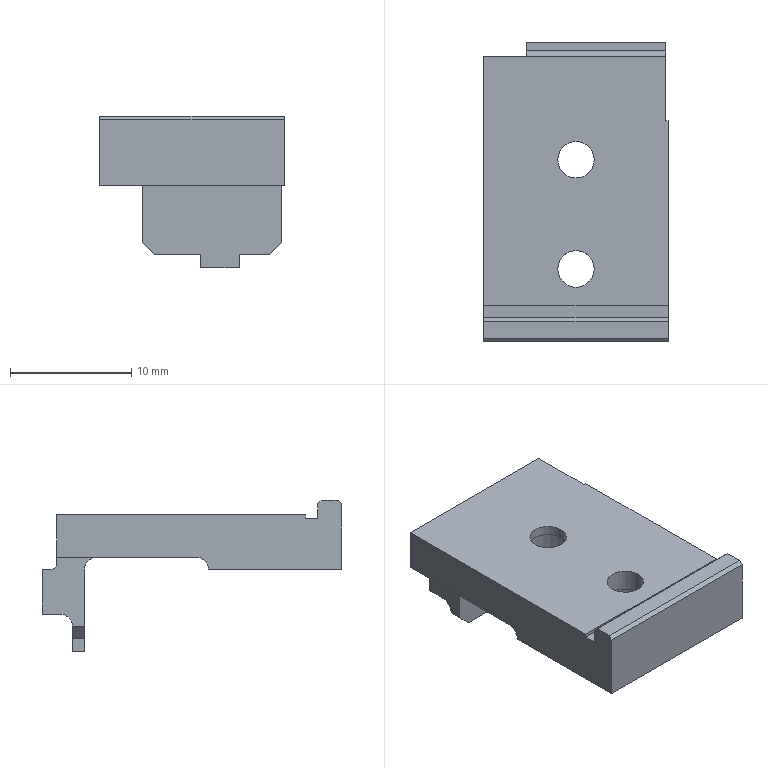Part | NX | 1 solid | 43 faces | box 15.2 x 24.7 x 12.5 mm | volume 1529 mm3 | plane 31 | cylinder 12 | commonest cylinder face diameters 3 x4 5 x4 2 x3 1 x1
STEP:
#1=CARTESIAN_POINT('',(-15.2,-12.7,1.));
#2=VERTEX_POINT('',#1);
#3=CARTESIAN_POINT('',(-15.2,-1.2,1.));
#4=VERTEX_POINT('',#3);
#5=CARTESIAN_POINT('',(-15.2,0.,1.));
#6=DIRECTION('',(0.,1.,0.));
#7=VECTOR('',#6,1000.);
#8=LINE('',#5,#7);
#9=EDGE_CURVE('',#2,#4,#8,.T.);
#10=ORIENTED_EDGE('',*,*,#9,.F.);
#11=CARTESIAN_POINT('',(-15.2,-13.7,0.));
#12=VERTEX_POINT('',#11);
#13=CARTESIAN_POINT('',(-15.2,-12.7,0.));
#14=DIRECTION('',(1.,0.,0.));
#15=DIRECTION('',(0.,-1.,0.));
#16=AXIS2_PLACEMENT_3D('',#13,#14,#15);
#17=CIRCLE('',#16,1.);
#18=EDGE_CURVE('',#2,#12,#17,.T.);
#19=ORIENTED_EDGE('',*,*,#18,.T.);
#20=CARTESIAN_POINT('',(-15.2,-24.7,0.));
#21=VERTEX_POINT('',#20);
#22=CARTESIAN_POINT('',(-15.2,0.,0.));
#23=DIRECTION('',(0.,1.,0.));
#24=VECTOR('',#23,1000.);
#25=LINE('',#22,#24);
#26=EDGE_CURVE('',#21,#12,#25,.T.);
#27=ORIENTED_EDGE('',*,*,#26,.F.);
#28=CARTESIAN_POINT('',(-15.2,-24.7,5.4));
#29=VERTEX_POINT('',#28);
#30=CARTESIAN_POINT('',(-15.2,-24.7,0.));
#31=DIRECTION('',(0.,0.,-1.));
#32=VECTOR('',#31,1000.);
#33=LINE('',#30,#32);
#34=EDGE_CURVE('',#29,#21,#33,.T.);
#35=ORIENTED_EDGE('',*,*,#34,.F.);
#36=CARTESIAN_POINT('',(-15.2,-24.4,5.7));
#37=VERTEX_POINT('',#36);
#38=CARTESIAN_POINT('',(-15.2,0.,30.1));
#39=DIRECTION('',(0.,0.7071,0.7071));
#40=VECTOR('',#39,1000.);
#41=LINE('',#38,#40);
#42=EDGE_CURVE('',#29,#37,#41,.T.);
#43=ORIENTED_EDGE('',*,*,#42,.T.);
#44=CARTESIAN_POINT('',(-15.2,-23.,5.7));
#45=VERTEX_POINT('',#44);
#46=CARTESIAN_POINT('',(-15.2,0.,5.7));
#47=DIRECTION('',(0.,1.,0.));
#48=VECTOR('',#47,1000.);
#49=LINE('',#46,#48);
#50=EDGE_CURVE('',#37,#45,#49,.T.);
#51=ORIENTED_EDGE('',*,*,#50,.T.);
#52=CARTESIAN_POINT('',(-15.2,-22.7,5.4));
#53=VERTEX_POINT('',#52);
#54=CARTESIAN_POINT('',(-15.2,0.,-17.3));
#55=DIRECTION('',(0.,-0.7071,0.7071));
#56=VECTOR('',#55,1000.);
#57=LINE('',#54,#56);
#58=EDGE_CURVE('',#53,#45,#57,.T.);
#59=ORIENTED_EDGE('',*,*,#58,.F.);
#60=CARTESIAN_POINT('',(-15.2,-22.7,4.2));
#61=VERTEX_POINT('',#60);
#62=CARTESIAN_POINT('',(-15.2,-22.7,0.));
#63=DIRECTION('',(0.,0.,-1.));
#64=VECTOR('',#63,1000.);
#65=LINE('',#62,#64);
#66=EDGE_CURVE('',#53,#61,#65,.T.);
#67=ORIENTED_EDGE('',*,*,#66,.T.);
#68=CARTESIAN_POINT('',(-15.2,-21.7,4.2));
#69=VERTEX_POINT('',#68);
#70=CARTESIAN_POINT('',(-15.2,0.,4.2));
#71=DIRECTION('',(0.,-1.,0.));
#72=VECTOR('',#71,1000.);
#73=LINE('',#70,#72);
#74=EDGE_CURVE('',#69,#61,#73,.T.);
#75=ORIENTED_EDGE('',*,*,#74,.F.);
#76=CARTESIAN_POINT('',(-15.2,-21.7,4.5));
#77=VERTEX_POINT('',#76);
#78=CARTESIAN_POINT('',(-15.2,-21.7,0.));
#79=DIRECTION('',(0.,0.,-1.));
#80=VECTOR('',#79,1000.);
#81=LINE('',#78,#80);
#82=EDGE_CURVE('',#77,#69,#81,.T.);
#83=ORIENTED_EDGE('',*,*,#82,.F.);
#84=CARTESIAN_POINT('',(-15.2,-1.2,4.5));
#85=VERTEX_POINT('',#84);
#86=CARTESIAN_POINT('',(-15.2,0.,4.5));
#87=DIRECTION('',(0.,-1.,0.));
#88=VECTOR('',#87,1000.);
#89=LINE('',#86,#88);
#90=EDGE_CURVE('',#85,#77,#89,.T.);
#91=ORIENTED_EDGE('',*,*,#90,.F.);
#92=CARTESIAN_POINT('',(-15.2,-1.2,0.));
#93=DIRECTION('',(0.,0.,1.));
#94=VECTOR('',#93,1000.);
#95=LINE('',#92,#94);
#96=EDGE_CURVE('',#4,#85,#95,.T.);
#97=ORIENTED_EDGE('',*,*,#96,.F.);
#98=EDGE_LOOP('',(#10,#19,#27,#35,#43,#51,#59,#67,#75,#83,#91,#97));
#99=FACE_BOUND('',#98,.T.);
#100=CARTESIAN_POINT('',(-15.2,0.,0.));
#101=DIRECTION('',(1.,0.,0.));
#102=DIRECTION('',(0.,1.,0.));
#103=AXIS2_PLACEMENT_3D('',#100,#101,#102);
#104=PLANE('',#103);
#105=ADVANCED_FACE('',(#99),#104,.F.);
#106=CARTESIAN_POINT('',(0.,-21.7,4.5));
#107=VERTEX_POINT('',#106);
#108=CARTESIAN_POINT('',(0.,-6.5,4.5));
#109=VERTEX_POINT('',#108);
#110=CARTESIAN_POINT('',(0.,0.,4.5));
#111=DIRECTION('',(0.,1.,0.));
#112=VECTOR('',#111,1000.);
#113=LINE('',#110,#112);
#114=EDGE_CURVE('',#107,#109,#113,.T.);
#115=ORIENTED_EDGE('',*,*,#114,.F.);
#116=CARTESIAN_POINT('',(0.,-21.7,4.2));
#117=VERTEX_POINT('',#116);
#118=CARTESIAN_POINT('',(0.,-21.7,0.));
#119=DIRECTION('',(0.,0.,1.));
#120=VECTOR('',#119,1000.);
#121=LINE('',#118,#120);
#122=EDGE_CURVE('',#117,#107,#121,.T.);
#123=ORIENTED_EDGE('',*,*,#122,.F.);
#124=CARTESIAN_POINT('',(0.,-22.7,4.2));
#125=VERTEX_POINT('',#124);
#126=CARTESIAN_POINT('',(0.,0.,4.2));
#127=DIRECTION('',(0.,1.,0.));
#128=VECTOR('',#127,1000.);
#129=LINE('',#126,#128);
#130=EDGE_CURVE('',#125,#117,#129,.T.);
#131=ORIENTED_EDGE('',*,*,#130,.F.);
#132=CARTESIAN_POINT('',(0.,-22.7,5.4));
#133=VERTEX_POINT('',#132);
#134=CARTESIAN_POINT('',(0.,-22.7,0.));
#135=DIRECTION('',(0.,0.,1.));
#136=VECTOR('',#135,1000.);
#137=LINE('',#134,#136);
#138=EDGE_CURVE('',#125,#133,#137,.T.);
#139=ORIENTED_EDGE('',*,*,#138,.T.);
#140=CARTESIAN_POINT('',(0.,-23.,5.7));
#141=VERTEX_POINT('',#140);
#142=CARTESIAN_POINT('',(0.,0.,-17.3));
#143=DIRECTION('',(0.,0.7071,-0.7071));
#144=VECTOR('',#143,1000.);
#145=LINE('',#142,#144);
#146=EDGE_CURVE('',#141,#133,#145,.T.);
#147=ORIENTED_EDGE('',*,*,#146,.F.);
#148=CARTESIAN_POINT('',(0.,-24.4,5.7));
#149=VERTEX_POINT('',#148);
#150=CARTESIAN_POINT('',(0.,0.,5.7));
#151=DIRECTION('',(0.,-1.,0.));
#152=VECTOR('',#151,1000.);
#153=LINE('',#150,#152);
#154=EDGE_CURVE('',#141,#149,#153,.T.);
#155=ORIENTED_EDGE('',*,*,#154,.T.);
#156=CARTESIAN_POINT('',(0.,-24.7,5.4));
#157=VERTEX_POINT('',#156);
#158=CARTESIAN_POINT('',(0.,0.,30.1));
#159=DIRECTION('',(0.,-0.7071,-0.7071));
#160=VECTOR('',#159,1000.);
#161=LINE('',#158,#160);
#162=EDGE_CURVE('',#149,#157,#161,.T.);
#163=ORIENTED_EDGE('',*,*,#162,.T.);
#164=CARTESIAN_POINT('',(0.,-24.7,0.));
#165=VERTEX_POINT('',#164);
#166=CARTESIAN_POINT('',(0.,-24.7,0.));
#167=DIRECTION('',(0.,0.,1.));
#168=VECTOR('',#167,1000.);
#169=LINE('',#166,#168);
#170=EDGE_CURVE('',#165,#157,#169,.T.);
#171=ORIENTED_EDGE('',*,*,#170,.F.);
#172=CARTESIAN_POINT('',(0.,-13.7,0.));
#173=VERTEX_POINT('',#172);
#174=CARTESIAN_POINT('',(0.,0.,0.));
#175=DIRECTION('',(0.,-1.,0.));
#176=VECTOR('',#175,1000.);
#177=LINE('',#174,#176);
#178=EDGE_CURVE('',#173,#165,#177,.T.);
#179=ORIENTED_EDGE('',*,*,#178,.F.);
#180=CARTESIAN_POINT('',(0.,-12.7,1.));
#181=VERTEX_POINT('',#180);
#182=CARTESIAN_POINT('',(0.,-12.7,0.));
#183=DIRECTION('',(1.,0.,0.));
#184=DIRECTION('',(0.,-1.,0.));
#185=AXIS2_PLACEMENT_3D('',#182,#183,#184);
#186=CIRCLE('',#185,1.);
#187=EDGE_CURVE('',#181,#173,#186,.T.);
#188=ORIENTED_EDGE('',*,*,#187,.F.);
#189=CARTESIAN_POINT('',(0.,-6.5,1.));
#190=VERTEX_POINT('',#189);
#191=CARTESIAN_POINT('',(0.,0.,1.));
#192=DIRECTION('',(0.,-1.,0.));
#193=VECTOR('',#192,1000.);
#194=LINE('',#191,#193);
#195=EDGE_CURVE('',#190,#181,#194,.T.);
#196=ORIENTED_EDGE('',*,*,#195,.F.);
#197=CARTESIAN_POINT('',(0.,-6.5,0.));
#198=DIRECTION('',(0.,0.,-1.));
#199=VECTOR('',#198,1000.);
#200=LINE('',#197,#199);
#201=EDGE_CURVE('',#109,#190,#200,.T.);
#202=ORIENTED_EDGE('',*,*,#201,.F.);
#203=EDGE_LOOP('',(#115,#123,#131,#139,#147,#155,#163,#171,#179,#188,#196,#202));
#204=FACE_BOUND('',#203,.T.);
#205=CARTESIAN_POINT('',(0.,-24.7,0.));
#206=DIRECTION('',(-1.,0.,0.));
#207=DIRECTION('',(0.,0.,1.));
#208=AXIS2_PLACEMENT_3D('',#205,#206,#207);
#209=PLANE('',#208);
#210=ADVANCED_FACE('',(#204),#209,.F.);
#211=CARTESIAN_POINT('',(-10.1,-18.7,2.7));
#212=VERTEX_POINT('',#211);
#213=CARTESIAN_POINT('',(-5.1,-18.7,2.7));
#214=VERTEX_POINT('',#213);
#215=CARTESIAN_POINT('',(-7.6,-18.7,2.7));
#216=DIRECTION('',(0.,0.,-1.));
#217=DIRECTION('',(-1.,0.,0.));
#218=AXIS2_PLACEMENT_3D('',#215,#216,#217);
#219=CIRCLE('',#218,2.5);
#220=EDGE_CURVE('',#212,#214,#219,.T.);
#221=ORIENTED_EDGE('',*,*,#220,.T.);
#222=CARTESIAN_POINT('',(-7.6,-18.7,2.7));
#223=DIRECTION('',(0.,0.,-1.));
#224=DIRECTION('',(-1.,0.,0.));
#225=AXIS2_PLACEMENT_3D('',#222,#223,#224);
#226=CIRCLE('',#225,2.5);
#227=EDGE_CURVE('',#214,#212,#226,.T.);
#228=ORIENTED_EDGE('',*,*,#227,.T.);
#229=EDGE_LOOP('',(#221,#228));
#230=FACE_BOUND('',#229,.T.);
#231=CARTESIAN_POINT('',(-6.1,-18.7,2.7));
#232=VERTEX_POINT('',#231);
#233=CARTESIAN_POINT('',(-9.1,-18.7,2.7));
#234=VERTEX_POINT('',#233);
#235=CARTESIAN_POINT('',(-7.6,-18.7,2.7));
#236=DIRECTION('',(0.,0.,-1.));
#237=DIRECTION('',(-1.,0.,0.));
#238=AXIS2_PLACEMENT_3D('',#235,#236,#237);
#239=CIRCLE('',#238,1.5);
#240=EDGE_CURVE('',#232,#234,#239,.T.);
#241=ORIENTED_EDGE('',*,*,#240,.F.);
#242=CARTESIAN_POINT('',(-7.6,-18.7,2.7));
#243=DIRECTION('',(0.,0.,-1.));
#244=DIRECTION('',(-1.,0.,0.));
#245=AXIS2_PLACEMENT_3D('',#242,#243,#244);
#246=CIRCLE('',#245,1.5);
#247=EDGE_CURVE('',#234,#232,#246,.T.);
#248=ORIENTED_EDGE('',*,*,#247,.F.);
#249=EDGE_LOOP('',(#241,#248));
#250=FACE_BOUND('',#249,.T.);
#251=CARTESIAN_POINT('',(-11.486,-5.492,2.7));
#252=DIRECTION('',(0.,0.,-1.));
#253=DIRECTION('',(0.,-1.,0.));
#254=AXIS2_PLACEMENT_3D('',#251,#252,#253);
#255=PLANE('',#254);
#256=ADVANCED_FACE('',(#230,#250),#255,.T.);
#257=CARTESIAN_POINT('',(-0.2,-4.5,1.));
#258=VERTEX_POINT('',#257);
#259=CARTESIAN_POINT('',(-11.7,-4.5,1.));
#260=VERTEX_POINT('',#259);
#261=CARTESIAN_POINT('',(0.,-4.5,1.));
#262=DIRECTION('',(-1.,0.,0.));
#263=VECTOR('',#262,1000.);
#264=LINE('',#261,#263);
#265=EDGE_CURVE('',#258,#260,#264,.T.);
#266=ORIENTED_EDGE('',*,*,#265,.F.);
#267=CARTESIAN_POINT('',(-0.2,-6.5,1.));
#268=VERTEX_POINT('',#267);
#269=CARTESIAN_POINT('',(-0.2,0.,1.));
#270=DIRECTION('',(0.,1.,0.));
#271=VECTOR('',#270,1000.);
#272=LINE('',#269,#271);
#273=EDGE_CURVE('',#268,#258,#272,.T.);
#274=ORIENTED_EDGE('',*,*,#273,.F.);
#275=CARTESIAN_POINT('',(0.,-6.5,1.));
#276=DIRECTION('',(-1.,0.,0.));
#277=VECTOR('',#276,1000.);
#278=LINE('',#275,#277);
#279=EDGE_CURVE('',#190,#268,#278,.T.);
#280=ORIENTED_EDGE('',*,*,#279,.F.);
#281=ORIENTED_EDGE('',*,*,#195,.T.);
#282=CARTESIAN_POINT('',(0.,-12.7,1.));
#283=DIRECTION('',(1.,0.,0.));
#284=VECTOR('',#283,1000.);
#285=LINE('',#282,#284);
#286=EDGE_CURVE('',#2,#181,#285,.T.);
#287=ORIENTED_EDGE('',*,*,#286,.F.);
#288=ORIENTED_EDGE('',*,*,#9,.T.);
#289=CARTESIAN_POINT('',(-11.7,-1.2,1.));
#290=VERTEX_POINT('',#289);
#291=CARTESIAN_POINT('',(0.,-1.2,1.));
#292=DIRECTION('',(-1.,0.,0.));
#293=VECTOR('',#292,1000.);
#294=LINE('',#291,#293);
#295=EDGE_CURVE('',#290,#4,#294,.T.);
#296=ORIENTED_EDGE('',*,*,#295,.F.);
#297=CARTESIAN_POINT('',(-11.7,0.,1.));
#298=DIRECTION('',(0.,1.,0.));
#299=VECTOR('',#298,1000.);
#300=LINE('',#297,#299);
#301=EDGE_CURVE('',#260,#290,#300,.T.);
#302=ORIENTED_EDGE('',*,*,#301,.F.);
#303=EDGE_LOOP('',(#266,#274,#280,#281,#287,#288,#296,#302));
#304=FACE_BOUND('',#303,.T.);
#305=CARTESIAN_POINT('',(-5.1,-9.7,1.));
#306=VERTEX_POINT('',#305);
#307=CARTESIAN_POINT('',(-10.1,-9.7,1.));
#308=VERTEX_POINT('',#307);
#309=CARTESIAN_POINT('',(-7.6,-9.7,1.));
#310=DIRECTION('',(0.,0.,-1.));
#311=DIRECTION('',(-1.,0.,0.));
#312=AXIS2_PLACEMENT_3D('',#309,#310,#311);
#313=CIRCLE('',#312,2.5);
#314=EDGE_CURVE('',#306,#308,#313,.T.);
#315=ORIENTED_EDGE('',*,*,#314,.F.);
#316=CARTESIAN_POINT('',(-7.6,-9.7,1.));
#317=DIRECTION('',(0.,0.,-1.));
#318=DIRECTION('',(-1.,0.,0.));
#319=AXIS2_PLACEMENT_3D('',#316,#317,#318);
#320=CIRCLE('',#319,2.5);
#321=EDGE_CURVE('',#308,#306,#320,.T.);
#322=ORIENTED_EDGE('',*,*,#321,.F.);
#323=EDGE_LOOP('',(#315,#322));
#324=FACE_BOUND('',#323,.T.);
#325=CARTESIAN_POINT('',(-11.724,-4.43,1.));
#326=DIRECTION('',(0.,0.,-1.));
#327=DIRECTION('',(0.,-1.,0.));
#328=AXIS2_PLACEMENT_3D('',#325,#326,#327);
#329=PLANE('',#328);
#330=ADVANCED_FACE('',(#304,#324),#329,.T.);
#331=CARTESIAN_POINT('',(-0.2,0.,-3.7));
#332=VERTEX_POINT('',#331);
#333=CARTESIAN_POINT('',(-0.2,-1.5,-3.7));
#334=VERTEX_POINT('',#333);
#335=CARTESIAN_POINT('',(-0.2,0.,-3.7));
#336=DIRECTION('',(0.,-1.,0.));
#337=VECTOR('',#336,1000.);
#338=LINE('',#335,#337);
#339=EDGE_CURVE('',#332,#334,#338,.T.);
#340=ORIENTED_EDGE('',*,*,#339,.F.);
#341=CARTESIAN_POINT('',(-0.2,0.,0.));
#342=VERTEX_POINT('',#341);
#343=CARTESIAN_POINT('',(-0.2,0.,0.));
#344=DIRECTION('',(0.,0.,-1.));
#345=VECTOR('',#344,1000.);
#346=LINE('',#343,#345);
#347=EDGE_CURVE('',#342,#332,#346,.T.);
#348=ORIENTED_EDGE('',*,*,#347,.F.);
#349=CARTESIAN_POINT('',(-0.2,-0.7,0.));
#350=VERTEX_POINT('',#349);
#351=CARTESIAN_POINT('',(-0.2,0.,0.));
#352=DIRECTION('',(0.,-1.,0.));
#353=VECTOR('',#352,1000.);
#354=LINE('',#351,#353);
#355=EDGE_CURVE('',#342,#350,#354,.T.);
#356=ORIENTED_EDGE('',*,*,#355,.T.);
#357=CARTESIAN_POINT('',(-0.2,-1.2,0.5));
#358=VERTEX_POINT('',#357);
#359=CARTESIAN_POINT('',(-0.2,-0.7,0.5));
#360=DIRECTION('',(-1.,0.,0.));
#361=DIRECTION('',(0.,1.,0.));
#362=AXIS2_PLACEMENT_3D('',#359,#360,#361);
#363=CIRCLE('',#362,0.5);
#364=EDGE_CURVE('',#350,#358,#363,.T.);
#365=ORIENTED_EDGE('',*,*,#364,.T.);
#366=CARTESIAN_POINT('',(-0.2,-1.2,4.5));
#367=VERTEX_POINT('',#366);
#368=CARTESIAN_POINT('',(-0.2,-1.2,0.));
#369=DIRECTION('',(0.,0.,1.));
#370=VECTOR('',#369,1000.);
#371=LINE('',#368,#370);
#372=EDGE_CURVE('',#358,#367,#371,.T.);
#373=ORIENTED_EDGE('',*,*,#372,.T.);
#374=CARTESIAN_POINT('',(-0.2,-6.5,4.5));
#375=VERTEX_POINT('',#374);
#376=CARTESIAN_POINT('',(-0.2,0.,4.5));
#377=DIRECTION('',(0.,-1.,0.));
#378=VECTOR('',#377,1000.);
#379=LINE('',#376,#378);
#380=EDGE_CURVE('',#367,#375,#379,.T.);
#381=ORIENTED_EDGE('',*,*,#380,.T.);
#382=CARTESIAN_POINT('',(-0.2,-6.5,0.));
#383=DIRECTION('',(0.,0.,1.));
#384=VECTOR('',#383,1000.);
#385=LINE('',#382,#384);
#386=EDGE_CURVE('',#268,#375,#385,.T.);
#387=ORIENTED_EDGE('',*,*,#386,.F.);
#388=ORIENTED_EDGE('',*,*,#273,.T.);
#389=CARTESIAN_POINT('',(-0.2,-3.5,0.));
#390=VERTEX_POINT('',#389);
#391=CARTESIAN_POINT('',(-0.2,-4.5,0.));
#392=DIRECTION('',(-1.,0.,0.));
#393=DIRECTION('',(0.,1.,0.));
#394=AXIS2_PLACEMENT_3D('',#391,#392,#393);
#395=CIRCLE('',#394,1.);
#396=EDGE_CURVE('',#258,#390,#395,.T.);
#397=ORIENTED_EDGE('',*,*,#396,.T.);
#398=CARTESIAN_POINT('',(-0.2,-3.5,-4.7));
#399=VERTEX_POINT('',#398);
#400=CARTESIAN_POINT('',(-0.2,-3.5,0.));
#401=DIRECTION('',(0.,0.,-1.));
#402=VECTOR('',#401,1000.);
#403=LINE('',#400,#402);
#404=EDGE_CURVE('',#390,#399,#403,.T.);
#405=ORIENTED_EDGE('',*,*,#404,.T.);
#406=CARTESIAN_POINT('',(-0.2,-2.5,-4.7));
#407=VERTEX_POINT('',#406);
#408=CARTESIAN_POINT('',(-0.2,0.,-4.7));
#409=DIRECTION('',(0.,1.,0.));
#410=VECTOR('',#409,1000.);
#411=LINE('',#408,#410);
#412=EDGE_CURVE('',#399,#407,#411,.T.);
#413=ORIENTED_EDGE('',*,*,#412,.T.);
#414=CARTESIAN_POINT('',(-0.2,-1.5,-4.7));
#415=DIRECTION('',(-1.,0.,0.));
#416=DIRECTION('',(0.,1.,0.));
#417=AXIS2_PLACEMENT_3D('',#414,#415,#416);
#418=CIRCLE('',#417,1.);
#419=EDGE_CURVE('',#407,#334,#418,.T.);
#420=ORIENTED_EDGE('',*,*,#419,.T.);
#421=EDGE_LOOP('',(#340,#348,#356,#365,#373,#381,#387,#388,#397,#405,#413,#420));
#422=FACE_BOUND('',#421,.T.);
#423=CARTESIAN_POINT('',(-0.2,-6.5,2.));
#424=DIRECTION('',(1.,0.,0.));
#425=DIRECTION('',(0.,1.,0.));
#426=AXIS2_PLACEMENT_3D('',#423,#424,#425);
#427=PLANE('',#426);
#428=ADVANCED_FACE('',(#422),#427,.T.);
#429=ORIENTED_EDGE('',*,*,#82,.T.);
#430=CARTESIAN_POINT('',(0.,-21.7,4.2));
#431=DIRECTION('',(1.,0.,0.));
#432=VECTOR('',#431,1000.);
#433=LINE('',#430,#432);
#434=EDGE_CURVE('',#69,#117,#433,.T.);
#435=ORIENTED_EDGE('',*,*,#434,.T.);
#436=ORIENTED_EDGE('',*,*,#122,.T.);
#437=CARTESIAN_POINT('',(0.,-21.7,4.5));
#438=DIRECTION('',(-1.,0.,0.));
#439=VECTOR('',#438,1000.);
#440=LINE('',#437,#439);
#441=EDGE_CURVE('',#107,#77,#440,.T.);
#442=ORIENTED_EDGE('',*,*,#441,.T.);
#443=EDGE_LOOP('',(#429,#435,#436,#442));
#444=FACE_BOUND('',#443,.T.);
#445=CARTESIAN_POINT('',(0.,-21.7,2.));
#446=DIRECTION('',(0.,-1.,0.));
#447=DIRECTION('',(0.,0.,-1.));
#448=AXIS2_PLACEMENT_3D('',#445,#446,#447);
#449=PLANE('',#448);
#450=ADVANCED_FACE('',(#444),#449,.T.);
#451=CARTESIAN_POINT('',(-11.7,-3.5,0.));
#452=VERTEX_POINT('',#451);
#453=CARTESIAN_POINT('',(-11.7,-3.5,-4.7));
#454=VERTEX_POINT('',#453);
#455=CARTESIAN_POINT('',(-11.7,-3.5,0.));
#456=DIRECTION('',(0.,0.,-1.));
#457=VECTOR('',#456,1000.);
#458=LINE('',#455,#457);
#459=EDGE_CURVE('',#452,#454,#458,.T.);
#460=ORIENTED_EDGE('',*,*,#459,.F.);
#461=CARTESIAN_POINT('',(-11.7,-4.5,0.));
#462=DIRECTION('',(-1.,0.,0.));
#463=DIRECTION('',(0.,1.,0.));
#464=AXIS2_PLACEMENT_3D('',#461,#462,#463);
#465=CIRCLE('',#464,1.);
#466=EDGE_CURVE('',#260,#452,#465,.T.);
#467=ORIENTED_EDGE('',*,*,#466,.F.);
#468=ORIENTED_EDGE('',*,*,#301,.T.);
#469=CARTESIAN_POINT('',(-11.7,-1.2,0.5));
#470=VERTEX_POINT('',#469);
#471=CARTESIAN_POINT('',(-11.7,-1.2,0.));
#472=DIRECTION('',(0.,0.,1.));
#473=VECTOR('',#472,1000.);
#474=LINE('',#471,#473);
#475=EDGE_CURVE('',#470,#290,#474,.T.);
#476=ORIENTED_EDGE('',*,*,#475,.F.);
#477=CARTESIAN_POINT('',(-11.7,-0.7,0.));
#478=VERTEX_POINT('',#477);
#479=CARTESIAN_POINT('',(-11.7,-0.7,0.5));
#480=DIRECTION('',(-1.,0.,0.));
#481=DIRECTION('',(0.,1.,0.));
#482=AXIS2_PLACEMENT_3D('',#479,#480,#481);
#483=CIRCLE('',#482,0.5);
#484=EDGE_CURVE('',#478,#470,#483,.T.);
#485=ORIENTED_EDGE('',*,*,#484,.F.);
#486=CARTESIAN_POINT('',(-11.7,0.,0.));
#487=VERTEX_POINT('',#486);
#488=CARTESIAN_POINT('',(-11.7,0.,0.));
#489=DIRECTION('',(0.,-1.,0.));
#490=VECTOR('',#489,1000.);
#491=LINE('',#488,#490);
#492=EDGE_CURVE('',#487,#478,#491,.T.);
#493=ORIENTED_EDGE('',*,*,#492,.F.);
#494=CARTESIAN_POINT('',(-11.7,0.,-3.7));
#495=VERTEX_POINT('',#494);
#496=CARTESIAN_POINT('',(-11.7,0.,0.));
#497=DIRECTION('',(0.,0.,-1.));
#498=VECTOR('',#497,1000.);
#499=LINE('',#496,#498);
#500=EDGE_CURVE('',#487,#495,#499,.T.);
#501=ORIENTED_EDGE('',*,*,#500,.T.);
#502=CARTESIAN_POINT('',(-11.7,-1.5,-3.7));
#503=VERTEX_POINT('',#502);
#504=CARTESIAN_POINT('',(-11.7,0.,-3.7));
#505=DIRECTION('',(0.,-1.,0.));
#506=VECTOR('',#505,1000.);
#507=LINE('',#504,#506);
#508=EDGE_CURVE('',#495,#503,#507,.T.);
#509=ORIENTED_EDGE('',*,*,#508,.T.);
#510=CARTESIAN_POINT('',(-11.7,-2.5,-4.7));
#511=VERTEX_POINT('',#510);
#512=CARTESIAN_POINT('',(-11.7,-1.5,-4.7));
#513=DIRECTION('',(-1.,0.,0.));
#514=DIRECTION('',(0.,1.,0.));
#515=AXIS2_PLACEMENT_3D('',#512,#513,#514);
#516=CIRCLE('',#515,1.);
#517=EDGE_CURVE('',#511,#503,#516,.T.);
#518=ORIENTED_EDGE('',*,*,#517,.F.);
#519=CARTESIAN_POINT('',(-11.7,0.,-4.7));
#520=DIRECTION('',(0.,-1.,0.));
#521=VECTOR('',#520,1000.);
#522=LINE('',#519,#521);
#523=EDGE_CURVE('',#511,#454,#522,.T.);
#524=ORIENTED_EDGE('',*,*,#523,.T.);
#525=EDGE_LOOP('',(#460,#467,#468,#476,#485,#493,#501,#509,#518,#524));
#526=FACE_BOUND('',#525,.T.);
#527=CARTESIAN_POINT('',(-11.7,-1.2,0.));
#528=DIRECTION('',(1.,0.,0.));
#529=DIRECTION('',(0.,1.,0.));
#530=AXIS2_PLACEMENT_3D('',#527,#528,#529);
#531=PLANE('',#530);
#532=ADVANCED_FACE('',(#526),#531,.F.);
#533=ORIENTED_EDGE('',*,*,#279,.T.);
#534=ORIENTED_EDGE('',*,*,#386,.T.);
#535=CARTESIAN_POINT('',(0.,-6.5,4.5));
#536=DIRECTION('',(1.,0.,0.));
#537=VECTOR('',#536,1000.);
#538=LINE('',#535,#537);
#539=EDGE_CURVE('',#375,#109,#538,.T.);
#540=ORIENTED_EDGE('',*,*,#539,.T.);
#541=ORIENTED_EDGE('',*,*,#201,.T.);
#542=EDGE_LOOP('',(#533,#534,#540,#541));
#543=FACE_BOUND('',#542,.T.);
#544=CARTESIAN_POINT('',(0.,-6.5,2.));
#545=DIRECTION('',(0.,1.,0.));
#546=DIRECTION('',(1.,0.,0.));
#547=AXIS2_PLACEMENT_3D('',#544,#545,#546);
#548=PLANE('',#547);
#549=ADVANCED_FACE('',(#543),#548,.T.);
#550=CARTESIAN_POINT('',(0.,-13.7,0.));
#551=DIRECTION('',(1.,0.,0.));
#552=VECTOR('',#551,1000.);
#553=LINE('',#550,#552);
#554=EDGE_CURVE('',#12,#173,#553,.T.);
#555=ORIENTED_EDGE('',*,*,#554,.T.);
#556=ORIENTED_EDGE('',*,*,#178,.T.);
#557=CARTESIAN_POINT('',(0.,-24.7,0.));
#558=DIRECTION('',(1.,0.,0.));
#559=VECTOR('',#558,1000.);
#560=LINE('',#557,#559);
#561=EDGE_CURVE('',#21,#165,#560,.T.);
#562=ORIENTED_EDGE('',*,*,#561,.F.);
#563=ORIENTED_EDGE('',*,*,#26,.T.);
#564=EDGE_LOOP('',(#555,#556,#562,#563));
#565=FACE_BOUND('',#564,.T.);
#566=CARTESIAN_POINT('',(-5.1,-18.7,0.));
#567=VERTEX_POINT('',#566);
#568=CARTESIAN_POINT('',(-10.1,-18.7,0.));
#569=VERTEX_POINT('',#568);
#570=CARTESIAN_POINT('',(-7.6,-18.7,0.));
#571=DIRECTION('',(0.,0.,-1.));
#572=DIRECTION('',(-1.,0.,0.));
#573=AXIS2_PLACEMENT_3D('',#570,#571,#572);
#574=CIRCLE('',#573,2.5);
#575=EDGE_CURVE('',#567,#569,#574,.T.);
#576=ORIENTED_EDGE('',*,*,#575,.F.);
#577=CARTESIAN_POINT('',(-7.6,-18.7,0.));
#578=DIRECTION('',(0.,0.,-1.));
#579=DIRECTION('',(-1.,0.,0.));
#580=AXIS2_PLACEMENT_3D('',#577,#578,#579);
#581=CIRCLE('',#580,2.5);
#582=EDGE_CURVE('',#569,#567,#581,.T.);
#583=ORIENTED_EDGE('',*,*,#582,.F.);
#584=EDGE_LOOP('',(#576,#583));
#585=FACE_BOUND('',#584,.T.);
#586=CARTESIAN_POINT('',(-11.977,-15.053,0.));
#587=DIRECTION('',(0.,0.,-1.));
#588=DIRECTION('',(0.,-1.,0.));
#589=AXIS2_PLACEMENT_3D('',#586,#587,#588);
#590=PLANE('',#589);
#591=ADVANCED_FACE('',(#565,#585),#590,.T.);
#592=ORIENTED_EDGE('',*,*,#355,.F.);
#593=CARTESIAN_POINT('',(0.,0.,0.));
#594=DIRECTION('',(1.,0.,0.));
#595=VECTOR('',#594,1000.);
#596=LINE('',#593,#595);
#597=EDGE_CURVE('',#487,#342,#596,.T.);
#598=ORIENTED_EDGE('',*,*,#597,.F.);
#599=ORIENTED_EDGE('',*,*,#492,.T.);
#600=CARTESIAN_POINT('',(0.,-0.7,0.));
#601=DIRECTION('',(-1.,0.,0.));
#602=VECTOR('',#601,1000.);
#603=LINE('',#600,#602);
#604=EDGE_CURVE('',#350,#478,#603,.T.);
#605=ORIENTED_EDGE('',*,*,#604,.F.);
#606=EDGE_LOOP('',(#592,#598,#599,#605));
#607=FACE_BOUND('',#606,.T.);
#608=CARTESIAN_POINT('',(-15.2,-1.2,0.));
#609=DIRECTION('',(0.,0.,1.));
#610=DIRECTION('',(1.,0.,0.));
#611=AXIS2_PLACEMENT_3D('',#608,#609,#610);
#612=PLANE('',#611);
#613=ADVANCED_FACE('',(#607),#612,.T.);
#614=CARTESIAN_POINT('',(0.,0.,-3.7));
#615=DIRECTION('',(1.,0.,0.));
#616=VECTOR('',#615,1000.);
#617=LINE('',#614,#616);
#618=EDGE_CURVE('',#495,#332,#617,.T.);
#619=ORIENTED_EDGE('',*,*,#618,.F.);
#620=ORIENTED_EDGE('',*,*,#500,.F.);
#621=ORIENTED_EDGE('',*,*,#597,.T.);
#622=ORIENTED_EDGE('',*,*,#347,.T.);
#623=EDGE_LOOP('',(#619,#620,#621,#622));
#624=FACE_BOUND('',#623,.T.);
#625=CARTESIAN_POINT('',(0.,0.,0.));
#626=DIRECTION('',(0.,-1.,0.));
#627=DIRECTION('',(0.,0.,-1.));
#628=AXIS2_PLACEMENT_3D('',#625,#626,#627);
#629=PLANE('',#628);
#630=ADVANCED_FACE('',(#624),#629,.F.);
#631=CARTESIAN_POINT('',(0.,-1.5,-3.7));
#632=DIRECTION('',(-1.,0.,0.));
#633=VECTOR('',#632,1000.);
#634=LINE('',#631,#633);
#635=EDGE_CURVE('',#334,#503,#634,.T.);
#636=ORIENTED_EDGE('',*,*,#635,.T.);
#637=ORIENTED_EDGE('',*,*,#508,.F.);
#638=ORIENTED_EDGE('',*,*,#618,.T.);
#639=ORIENTED_EDGE('',*,*,#339,.T.);
#640=EDGE_LOOP('',(#636,#637,#638,#639));
#641=FACE_BOUND('',#640,.T.);
#642=CARTESIAN_POINT('',(0.,0.,-3.7));
#643=DIRECTION('',(0.,0.,1.));
#644=DIRECTION('',(1.,0.,0.));
#645=AXIS2_PLACEMENT_3D('',#642,#643,#644);
#646=PLANE('',#645);
#647=ADVANCED_FACE('',(#641),#646,.F.);
#648=CARTESIAN_POINT('',(0.,-22.7,4.2));
#649=DIRECTION('',(1.,0.,0.));
#650=VECTOR('',#649,1000.);
#651=LINE('',#648,#650);
#652=EDGE_CURVE('',#61,#125,#651,.T.);
#653=ORIENTED_EDGE('',*,*,#652,.T.);
#654=ORIENTED_EDGE('',*,*,#130,.T.);
#655=ORIENTED_EDGE('',*,*,#434,.F.);
#656=ORIENTED_EDGE('',*,*,#74,.T.);
#657=EDGE_LOOP('',(#653,#654,#655,#656));
#658=FACE_BOUND('',#657,.T.);
#659=CARTESIAN_POINT('',(0.,-21.7,4.2));
#660=DIRECTION('',(0.,0.,1.));
#661=DIRECTION('',(1.,0.,0.));
#662=AXIS2_PLACEMENT_3D('',#659,#660,#661);
#663=PLANE('',#662);
#664=ADVANCED_FACE('',(#658),#663,.T.);
#665=CARTESIAN_POINT('',(-3.7,-3.5,-6.8));
#666=VERTEX_POINT('',#665);
#667=CARTESIAN_POINT('',(-3.7,-3.,-6.8));
#668=VERTEX_POINT('',#667);
#669=CARTESIAN_POINT('',(-3.7,0.,-6.8));
#670=DIRECTION('',(0.,1.,0.));
#671=VECTOR('',#670,1000.);
#672=LINE('',#669,#671);
#673=EDGE_CURVE('',#666,#668,#672,.T.);
#674=ORIENTED_EDGE('',*,*,#673,.F.);
#675=CARTESIAN_POINT('',(-6.9,-3.5,-6.8));
#676=VERTEX_POINT('',#675);
#677=CARTESIAN_POINT('',(0.,-3.5,-6.8));
#678=DIRECTION('',(-1.,0.,0.));
#679=VECTOR('',#678,1000.);
#680=LINE('',#677,#679);
#681=EDGE_CURVE('',#666,#676,#680,.T.);
#682=ORIENTED_EDGE('',*,*,#681,.T.);
#683=CARTESIAN_POINT('',(-6.9,-2.5,-6.8));
#684=VERTEX_POINT('',#683);
#685=CARTESIAN_POINT('',(-6.9,0.,-6.8));
#686=DIRECTION('',(0.,-1.,0.));
#687=VECTOR('',#686,1000.);
#688=LINE('',#685,#687);
#689=EDGE_CURVE('',#684,#676,#688,.T.);
#690=ORIENTED_EDGE('',*,*,#689,.F.);
#691=CARTESIAN_POINT('',(-4.7,-2.5,-6.8));
#692=VERTEX_POINT('',#691);
#693=CARTESIAN_POINT('',(0.,-2.5,-6.8));
#694=DIRECTION('',(-1.,0.,0.));
#695=VECTOR('',#694,1000.);
#696=LINE('',#693,#695);
#697=EDGE_CURVE('',#692,#684,#696,.T.);
#698=ORIENTED_EDGE('',*,*,#697,.F.);
#699=CARTESIAN_POINT('',(0.,-4.85,-6.8));
#700=DIRECTION('',(0.8944,-0.4472,0.));
#701=VECTOR('',#700,1000.);
#702=LINE('',#699,#701);
#703=EDGE_CURVE('',#692,#668,#702,.T.);
#704=ORIENTED_EDGE('',*,*,#703,.T.);
#705=EDGE_LOOP('',(#674,#682,#690,#698,#704));
#706=FACE_BOUND('',#705,.T.);
#707=CARTESIAN_POINT('',(-4.459,-2.381,-6.8));
#708=DIRECTION('',(0.,0.,-1.));
#709=DIRECTION('',(0.,-1.,0.));
#710=AXIS2_PLACEMENT_3D('',#707,#708,#709);
#711=PLANE('',#710);
#712=ADVANCED_FACE('',(#706),#711,.T.);
#713=CARTESIAN_POINT('',(0.,-1.2,0.5));
#714=DIRECTION('',(-1.,0.,0.));
#715=VECTOR('',#714,1000.);
#716=LINE('',#713,#715);
#717=EDGE_CURVE('',#358,#470,#716,.T.);
#718=ORIENTED_EDGE('',*,*,#717,.T.);
#719=ORIENTED_EDGE('',*,*,#475,.T.);
#720=ORIENTED_EDGE('',*,*,#295,.T.);
#721=ORIENTED_EDGE('',*,*,#96,.T.);
#722=CARTESIAN_POINT('',(0.,-1.2,4.5));
#723=DIRECTION('',(1.,0.,0.));
#724=VECTOR('',#723,1000.);
#725=LINE('',#722,#724);
#726=EDGE_CURVE('',#85,#367,#725,.T.);
#727=ORIENTED_EDGE('',*,*,#726,.T.);
#728=ORIENTED_EDGE('',*,*,#372,.F.);
#729=EDGE_LOOP('',(#718,#719,#720,#721,#727,#728));
#730=FACE_BOUND('',#729,.T.);
#731=CARTESIAN_POINT('',(-15.2,-1.2,2.));
#732=DIRECTION('',(0.,1.,0.));
#733=DIRECTION('',(1.,0.,0.));
#734=AXIS2_PLACEMENT_3D('',#731,#732,#733);
#735=PLANE('',#734);
#736=ADVANCED_FACE('',(#730),#735,.T.);
#737=ORIENTED_EDGE('',*,*,#286,.T.);
#738=ORIENTED_EDGE('',*,*,#187,.T.);
#739=ORIENTED_EDGE('',*,*,#554,.F.);
#740=ORIENTED_EDGE('',*,*,#18,.F.);
#741=EDGE_LOOP('',(#737,#738,#739,#740));
#742=FACE_BOUND('',#741,.T.);
#743=CARTESIAN_POINT('',(0.,-12.7,0.));
#744=DIRECTION('',(1.,0.,0.));
#745=DIRECTION('',(0.,-1.,0.));
#746=AXIS2_PLACEMENT_3D('',#743,#744,#745);
#747=CYLINDRICAL_SURFACE('',#746,1.);
#748=ADVANCED_FACE('',(#742),#747,.F.);
#749=CARTESIAN_POINT('',(0.,-23.,5.7));
#750=DIRECTION('',(-1.,0.,0.));
#751=VECTOR('',#750,1000.);
#752=LINE('',#749,#751);
#753=EDGE_CURVE('',#141,#45,#752,.T.);
#754=ORIENTED_EDGE('',*,*,#753,.T.);
#755=ORIENTED_EDGE('',*,*,#50,.F.);
#756=CARTESIAN_POINT('',(0.,-24.4,5.7));
#757=DIRECTION('',(-1.,0.,0.));
#758=VECTOR('',#757,1000.);
#759=LINE('',#756,#758);
#760=EDGE_CURVE('',#149,#37,#759,.T.);
#761=ORIENTED_EDGE('',*,*,#760,.F.);
#762=ORIENTED_EDGE('',*,*,#154,.F.);
#763=EDGE_LOOP('',(#754,#755,#761,#762));
#764=FACE_BOUND('',#763,.T.);
#765=CARTESIAN_POINT('',(0.,-22.7,5.7));
#766=DIRECTION('',(0.,0.,-1.));
#767=DIRECTION('',(0.,-1.,0.));
#768=AXIS2_PLACEMENT_3D('',#765,#766,#767);
#769=PLANE('',#768);
#770=ADVANCED_FACE('',(#764),#769,.F.);
#771=ORIENTED_EDGE('',*,*,#652,.F.);
#772=ORIENTED_EDGE('',*,*,#66,.F.);
#773=CARTESIAN_POINT('',(0.,-22.7,5.4));
#774=DIRECTION('',(1.,0.,0.));
#775=VECTOR('',#774,1000.);
#776=LINE('',#773,#775);
#777=EDGE_CURVE('',#53,#133,#776,.T.);
#778=ORIENTED_EDGE('',*,*,#777,.T.);
#779=ORIENTED_EDGE('',*,*,#138,.F.);
#780=EDGE_LOOP('',(#771,#772,#778,#779));
#781=FACE_BOUND('',#780,.T.);
#782=CARTESIAN_POINT('',(0.,-22.7,2.));
#783=DIRECTION('',(0.,-1.,0.));
#784=DIRECTION('',(0.,0.,-1.));
#785=AXIS2_PLACEMENT_3D('',#782,#783,#784);
#786=PLANE('',#785);
#787=ADVANCED_FACE('',(#781),#786,.F.);
#788=ORIENTED_EDGE('',*,*,#753,.F.);
#789=ORIENTED_EDGE('',*,*,#146,.T.);
#790=ORIENTED_EDGE('',*,*,#777,.F.);
#791=ORIENTED_EDGE('',*,*,#58,.T.);
#792=EDGE_LOOP('',(#788,#789,#790,#791));
#793=FACE_BOUND('',#792,.T.);
#794=CARTESIAN_POINT('',(-7.6,-22.85,5.55));
#795=DIRECTION('',(0.,0.7071,0.7071));
#796=DIRECTION('',(1.,0.,0.));
#797=AXIS2_PLACEMENT_3D('',#794,#795,#796);
#798=PLANE('',#797);
#799=ADVANCED_FACE('',(#793),#798,.T.);
#800=ORIENTED_EDGE('',*,*,#220,.F.);
#801=CARTESIAN_POINT('',(-10.1,-18.7,0.));
#802=DIRECTION('',(0.,0.,-1.));
#803=VECTOR('',#802,1000.);
#804=LINE('',#801,#803);
#805=EDGE_CURVE('',#569,#212,#804,.F.);
#806=ORIENTED_EDGE('',*,*,#805,.F.);
#807=ORIENTED_EDGE('',*,*,#582,.T.);
#808=CARTESIAN_POINT('',(-5.1,-18.7,0.));
#809=DIRECTION('',(0.,0.,-1.));
#810=VECTOR('',#809,1000.);
#811=LINE('',#808,#810);
#812=EDGE_CURVE('',#567,#214,#811,.F.);
#813=ORIENTED_EDGE('',*,*,#812,.T.);
#814=EDGE_LOOP('',(#800,#806,#807,#813));
#815=FACE_BOUND('',#814,.T.);
#816=CARTESIAN_POINT('',(-7.6,-18.7,0.));
#817=DIRECTION('',(0.,0.,-1.));
#818=DIRECTION('',(-1.,0.,0.));
#819=AXIS2_PLACEMENT_3D('',#816,#817,#818);
#820=CYLINDRICAL_SURFACE('',#819,2.5);
#821=ADVANCED_FACE('',(#815),#820,.F.);
#822=CARTESIAN_POINT('',(-5.1,-9.7,3.7));
#823=VERTEX_POINT('',#822);
#824=CARTESIAN_POINT('',(-10.1,-9.7,3.7));
#825=VERTEX_POINT('',#824);
#826=CARTESIAN_POINT('',(-7.6,-9.7,3.7));
#827=DIRECTION('',(0.,0.,-1.));
#828=DIRECTION('',(-1.,0.,0.));
#829=AXIS2_PLACEMENT_3D('',#826,#827,#828);
#830=CIRCLE('',#829,2.5);
#831=EDGE_CURVE('',#823,#825,#830,.T.);
#832=ORIENTED_EDGE('',*,*,#831,.F.);
#833=CARTESIAN_POINT('',(-5.1,-9.7,0.));
#834=DIRECTION('',(0.,0.,-1.));
#835=VECTOR('',#834,1000.);
#836=LINE('',#833,#835);
#837=EDGE_CURVE('',#306,#823,#836,.F.);
#838=ORIENTED_EDGE('',*,*,#837,.F.);
#839=ORIENTED_EDGE('',*,*,#314,.T.);
#840=CARTESIAN_POINT('',(-10.1,-9.7,0.));
#841=DIRECTION('',(0.,0.,-1.));
#842=VECTOR('',#841,1000.);
#843=LINE('',#840,#842);
#844=EDGE_CURVE('',#308,#825,#843,.F.);
#845=ORIENTED_EDGE('',*,*,#844,.T.);
#846=EDGE_LOOP('',(#832,#838,#839,#845));
#847=FACE_BOUND('',#846,.T.);
#848=CARTESIAN_POINT('',(-7.6,-9.7,0.));
#849=DIRECTION('',(0.,0.,-1.));
#850=DIRECTION('',(-1.,0.,0.));
#851=AXIS2_PLACEMENT_3D('',#848,#849,#850);
#852=CYLINDRICAL_SURFACE('',#851,2.5);
#853=ADVANCED_FACE('',(#847),#852,.F.);
#854=CARTESIAN_POINT('',(0.,-24.7,5.4));
#855=DIRECTION('',(1.,0.,0.));
#856=VECTOR('',#855,1000.);
#857=LINE('',#854,#856);
#858=EDGE_CURVE('',#29,#157,#857,.T.);
#859=ORIENTED_EDGE('',*,*,#858,.T.);
#860=ORIENTED_EDGE('',*,*,#162,.F.);
#861=ORIENTED_EDGE('',*,*,#760,.T.);
#862=ORIENTED_EDGE('',*,*,#42,.F.);
#863=EDGE_LOOP('',(#859,#860,#861,#862));
#864=FACE_BOUND('',#863,.T.);
#865=CARTESIAN_POINT('',(-7.6,-24.55,5.55));
#866=DIRECTION('',(0.,0.7071,-0.7071));
#867=DIRECTION('',(-1.,0.,0.));
#868=AXIS2_PLACEMENT_3D('',#865,#866,#867);
#869=PLANE('',#868);
#870=ADVANCED_FACE('',(#864),#869,.F.);
#871=CARTESIAN_POINT('',(-9.1,-9.7,3.7));
#872=VERTEX_POINT('',#871);
#873=CARTESIAN_POINT('',(-6.1,-9.7,3.7));
#874=VERTEX_POINT('',#873);
#875=CARTESIAN_POINT('',(-7.6,-9.7,3.7));
#876=DIRECTION('',(0.,0.,-1.));
#877=DIRECTION('',(-1.,0.,0.));
#878=AXIS2_PLACEMENT_3D('',#875,#876,#877);
#879=CIRCLE('',#878,1.5);
#880=EDGE_CURVE('',#872,#874,#879,.T.);
#881=ORIENTED_EDGE('',*,*,#880,.T.);
#882=CARTESIAN_POINT('',(-6.1,-9.7,4.5));
#883=VERTEX_POINT('',#882);
#884=CARTESIAN_POINT('',(-6.1,-9.7,5.45));
#885=DIRECTION('',(0.,0.,-1.));
#886=VECTOR('',#885,1000.);
#887=LINE('',#884,#886);
#888=EDGE_CURVE('',#883,#874,#887,.T.);
#889=ORIENTED_EDGE('',*,*,#888,.F.);
#890=CARTESIAN_POINT('',(-9.1,-9.7,4.5));
#891=VERTEX_POINT('',#890);
#892=CARTESIAN_POINT('',(-7.6,-9.7,4.5));
#893=DIRECTION('',(0.,0.,-1.));
#894=DIRECTION('',(-1.,0.,0.));
#895=AXIS2_PLACEMENT_3D('',#892,#893,#894);
#896=CIRCLE('',#895,1.5);
#897=EDGE_CURVE('',#891,#883,#896,.T.);
#898=ORIENTED_EDGE('',*,*,#897,.F.);
#899=CARTESIAN_POINT('',(-9.1,-9.7,5.45));
#900=DIRECTION('',(0.,0.,-1.));
#901=VECTOR('',#900,1000.);
#902=LINE('',#899,#901);
#903=EDGE_CURVE('',#891,#872,#902,.T.);
#904=ORIENTED_EDGE('',*,*,#903,.T.);
#905=EDGE_LOOP('',(#881,#889,#898,#904));
#906=FACE_BOUND('',#905,.T.);
#907=CARTESIAN_POINT('',(-7.6,-9.7,5.45));
#908=DIRECTION('',(0.,0.,-1.));
#909=DIRECTION('',(-1.,0.,0.));
#910=AXIS2_PLACEMENT_3D('',#907,#908,#909);
#911=CYLINDRICAL_SURFACE('',#910,1.5);
#912=ADVANCED_FACE('',(#906),#911,.F.);
#913=ORIENTED_EDGE('',*,*,#240,.T.);
#914=CARTESIAN_POINT('',(-9.1,-18.7,4.5));
#915=VERTEX_POINT('',#914);
#916=CARTESIAN_POINT('',(-9.1,-18.7,5.45));
#917=DIRECTION('',(0.,0.,-1.));
#918=VECTOR('',#917,1000.);
#919=LINE('',#916,#918);
#920=EDGE_CURVE('',#234,#915,#919,.F.);
#921=ORIENTED_EDGE('',*,*,#920,.T.);
#922=CARTESIAN_POINT('',(-6.1,-18.7,4.5));
#923=VERTEX_POINT('',#922);
#924=CARTESIAN_POINT('',(-7.6,-18.7,4.5));
#925=DIRECTION('',(0.,0.,-1.));
#926=DIRECTION('',(-1.,0.,0.));
#927=AXIS2_PLACEMENT_3D('',#924,#925,#926);
#928=CIRCLE('',#927,1.5);
#929=EDGE_CURVE('',#923,#915,#928,.T.);
#930=ORIENTED_EDGE('',*,*,#929,.F.);
#931=CARTESIAN_POINT('',(-6.1,-18.7,5.45));
#932=DIRECTION('',(0.,0.,-1.));
#933=VECTOR('',#932,1000.);
#934=LINE('',#931,#933);
#935=EDGE_CURVE('',#232,#923,#934,.F.);
#936=ORIENTED_EDGE('',*,*,#935,.F.);
#937=EDGE_LOOP('',(#913,#921,#930,#936));
#938=FACE_BOUND('',#937,.T.);
#939=CARTESIAN_POINT('',(-7.6,-18.7,5.45));
#940=DIRECTION('',(0.,0.,-1.));
#941=DIRECTION('',(-1.,0.,0.));
#942=AXIS2_PLACEMENT_3D('',#939,#940,#941);
#943=CYLINDRICAL_SURFACE('',#942,1.5);
#944=ADVANCED_FACE('',(#938),#943,.F.);
#945=ORIENTED_EDGE('',*,*,#380,.F.);
#946=ORIENTED_EDGE('',*,*,#726,.F.);
#947=ORIENTED_EDGE('',*,*,#90,.T.);
#948=ORIENTED_EDGE('',*,*,#441,.F.);
#949=ORIENTED_EDGE('',*,*,#114,.T.);
#950=ORIENTED_EDGE('',*,*,#539,.F.);
#951=EDGE_LOOP('',(#945,#946,#947,#948,#949,#950));
#952=FACE_BOUND('',#951,.T.);
#953=CARTESIAN_POINT('',(-7.6,-9.7,4.5));
#954=DIRECTION('',(0.,0.,-1.));
#955=DIRECTION('',(-1.,0.,0.));
#956=AXIS2_PLACEMENT_3D('',#953,#954,#955);
#957=CIRCLE('',#956,1.5);
#958=EDGE_CURVE('',#883,#891,#957,.T.);
#959=ORIENTED_EDGE('',*,*,#958,.T.);
#960=ORIENTED_EDGE('',*,*,#897,.T.);
#961=EDGE_LOOP('',(#959,#960));
#962=FACE_BOUND('',#961,.T.);
#963=CARTESIAN_POINT('',(-7.6,-18.7,4.5));
#964=DIRECTION('',(0.,0.,-1.));
#965=DIRECTION('',(-1.,0.,0.));
#966=AXIS2_PLACEMENT_3D('',#963,#964,#965);
#967=CIRCLE('',#966,1.5);
#968=EDGE_CURVE('',#915,#923,#967,.T.);
#969=ORIENTED_EDGE('',*,*,#968,.T.);
#970=ORIENTED_EDGE('',*,*,#929,.T.);
#971=EDGE_LOOP('',(#969,#970));
#972=FACE_BOUND('',#971,.T.);
#973=CARTESIAN_POINT('',(0.,0.,4.5));
#974=DIRECTION('',(0.,0.,1.));
#975=DIRECTION('',(1.,0.,0.));
#976=AXIS2_PLACEMENT_3D('',#973,#974,#975);
#977=PLANE('',#976);
#978=ADVANCED_FACE('',(#952,#962,#972),#977,.T.);
#979=ORIENTED_EDGE('',*,*,#831,.T.);
#980=CARTESIAN_POINT('',(-7.6,-9.7,3.7));
#981=DIRECTION('',(0.,0.,-1.));
#982=DIRECTION('',(-1.,0.,0.));
#983=AXIS2_PLACEMENT_3D('',#980,#981,#982);
#984=CIRCLE('',#983,2.5);
#985=EDGE_CURVE('',#825,#823,#984,.T.);
#986=ORIENTED_EDGE('',*,*,#985,.T.);
#987=EDGE_LOOP('',(#979,#986));
#988=FACE_BOUND('',#987,.T.);
#989=ORIENTED_EDGE('',*,*,#880,.F.);
#990=CARTESIAN_POINT('',(-7.6,-9.7,3.7));
#991=DIRECTION('',(0.,0.,-1.));
#992=DIRECTION('',(-1.,0.,0.));
#993=AXIS2_PLACEMENT_3D('',#990,#991,#992);
#994=CIRCLE('',#993,1.5);
#995=EDGE_CURVE('',#874,#872,#994,.T.);
#996=ORIENTED_EDGE('',*,*,#995,.F.);
#997=EDGE_LOOP('',(#989,#996));
#998=FACE_BOUND('',#997,.T.);
#999=CARTESIAN_POINT('',(-11.486,-5.592,3.7));
#1000=DIRECTION('',(0.,0.,-1.));
#1001=DIRECTION('',(0.,-1.,0.));
#1002=AXIS2_PLACEMENT_3D('',#999,#1000,#1001);
#1003=PLANE('',#1002);
#1004=ADVANCED_FACE('',(#988,#998),#1003,.T.);
#1005=ORIENTED_EDGE('',*,*,#717,.F.);
#1006=ORIENTED_EDGE('',*,*,#364,.F.);
#1007=ORIENTED_EDGE('',*,*,#604,.T.);
#1008=ORIENTED_EDGE('',*,*,#484,.T.);
#1009=EDGE_LOOP('',(#1005,#1006,#1007,#1008));
#1010=FACE_BOUND('',#1009,.T.);
#1011=CARTESIAN_POINT('',(0.,-0.7,0.5));
#1012=DIRECTION('',(-1.,0.,0.));
#1013=DIRECTION('',(0.,1.,0.));
#1014=AXIS2_PLACEMENT_3D('',#1011,#1012,#1013);
#1015=CYLINDRICAL_SURFACE('',#1014,0.5);
#1016=ADVANCED_FACE('',(#1010),#1015,.F.);
#1017=ORIENTED_EDGE('',*,*,#34,.T.);
#1018=ORIENTED_EDGE('',*,*,#561,.T.);
#1019=ORIENTED_EDGE('',*,*,#170,.T.);
#1020=ORIENTED_EDGE('',*,*,#858,.F.);
#1021=EDGE_LOOP('',(#1017,#1018,#1019,#1020));
#1022=FACE_BOUND('',#1021,.T.);
#1023=CARTESIAN_POINT('',(-15.2,-24.7,1.));
#1024=DIRECTION('',(0.,-1.,0.));
#1025=DIRECTION('',(0.,0.,-1.));
#1026=AXIS2_PLACEMENT_3D('',#1023,#1024,#1025);
#1027=PLANE('',#1026);
#1028=ADVANCED_FACE('',(#1022),#1027,.T.);
#1029=ORIENTED_EDGE('',*,*,#265,.T.);
#1030=ORIENTED_EDGE('',*,*,#466,.T.);
#1031=CARTESIAN_POINT('',(0.,-3.5,0.));
#1032=DIRECTION('',(-1.,0.,0.));
#1033=VECTOR('',#1032,1000.);
#1034=LINE('',#1031,#1033);
#1035=EDGE_CURVE('',#390,#452,#1034,.T.);
#1036=ORIENTED_EDGE('',*,*,#1035,.F.);
#1037=ORIENTED_EDGE('',*,*,#396,.F.);
#1038=EDGE_LOOP('',(#1029,#1030,#1036,#1037));
#1039=FACE_BOUND('',#1038,.T.);
#1040=CARTESIAN_POINT('',(0.,-4.5,0.));
#1041=DIRECTION('',(-1.,0.,0.));
#1042=DIRECTION('',(0.,1.,0.));
#1043=AXIS2_PLACEMENT_3D('',#1040,#1041,#1042);
#1044=CYLINDRICAL_SURFACE('',#1043,1.);
#1045=ADVANCED_FACE('',(#1039),#1044,.F.);
#1046=ORIENTED_EDGE('',*,*,#459,.T.);
#1047=CARTESIAN_POINT('',(-10.7,-3.5,-5.7));
#1048=VERTEX_POINT('',#1047);
#1049=CARTESIAN_POINT('',(-16.4,-3.5,0.));
#1050=DIRECTION('',(0.7071,0.,-0.7071));
#1051=VECTOR('',#1050,1000.);
#1052=LINE('',#1049,#1051);
#1053=EDGE_CURVE('',#454,#1048,#1052,.T.);
#1054=ORIENTED_EDGE('',*,*,#1053,.T.);
#1055=CARTESIAN_POINT('',(-6.9,-3.5,-5.7));
#1056=VERTEX_POINT('',#1055);
#1057=CARTESIAN_POINT('',(0.,-3.5,-5.7));
#1058=DIRECTION('',(1.,0.,0.));
#1059=VECTOR('',#1058,1000.);
#1060=LINE('',#1057,#1059);
#1061=EDGE_CURVE('',#1048,#1056,#1060,.T.);
#1062=ORIENTED_EDGE('',*,*,#1061,.T.);
#1063=CARTESIAN_POINT('',(-6.9,-3.5,0.));
#1064=DIRECTION('',(0.,0.,1.));
#1065=VECTOR('',#1064,1000.);
#1066=LINE('',#1063,#1065);
#1067=EDGE_CURVE('',#676,#1056,#1066,.T.);
#1068=ORIENTED_EDGE('',*,*,#1067,.F.);
#1069=ORIENTED_EDGE('',*,*,#681,.F.);
#1070=CARTESIAN_POINT('',(-3.7,-3.5,-5.7));
#1071=VERTEX_POINT('',#1070);
#1072=CARTESIAN_POINT('',(-3.7,-3.5,0.));
#1073=DIRECTION('',(0.,0.,-1.));
#1074=VECTOR('',#1073,1000.);
#1075=LINE('',#1072,#1074);
#1076=EDGE_CURVE('',#1071,#666,#1075,.T.);
#1077=ORIENTED_EDGE('',*,*,#1076,.F.);
#1078=CARTESIAN_POINT('',(-1.2,-3.5,-5.7));
#1079=VERTEX_POINT('',#1078);
#1080=CARTESIAN_POINT('',(0.,-3.5,-5.7));
#1081=DIRECTION('',(1.,0.,0.));
#1082=VECTOR('',#1081,1000.);
#1083=LINE('',#1080,#1082);
#1084=EDGE_CURVE('',#1071,#1079,#1083,.T.);
#1085=ORIENTED_EDGE('',*,*,#1084,.T.);
#1086=CARTESIAN_POINT('',(0.,-3.5,-4.5));
#1087=DIRECTION('',(-0.7071,0.,-0.7071));
#1088=VECTOR('',#1087,1000.);
#1089=LINE('',#1086,#1088);
#1090=EDGE_CURVE('',#399,#1079,#1089,.T.);
#1091=ORIENTED_EDGE('',*,*,#1090,.F.);
#1092=ORIENTED_EDGE('',*,*,#404,.F.);
#1093=ORIENTED_EDGE('',*,*,#1035,.T.);
#1094=EDGE_LOOP('',(#1046,#1054,#1062,#1068,#1069,#1077,#1085,#1091,#1092,#1093));
#1095=FACE_BOUND('',#1094,.T.);
#1096=CARTESIAN_POINT('',(-11.7,-3.5,-3.7));
#1097=DIRECTION('',(0.,-1.,0.));
#1098=DIRECTION('',(0.,0.,-1.));
#1099=AXIS2_PLACEMENT_3D('',#1096,#1097,#1098);
#1100=PLANE('',#1099);
#1101=ADVANCED_FACE('',(#1095),#1100,.T.);
#1102=CARTESIAN_POINT('',(-4.7,-2.5,-5.7));
#1103=VERTEX_POINT('',#1102);
#1104=CARTESIAN_POINT('',(-4.7,-2.5,0.));
#1105=DIRECTION('',(0.,0.,1.));
#1106=VECTOR('',#1105,1000.);
#1107=LINE('',#1104,#1106);
#1108=EDGE_CURVE('',#692,#1103,#1107,.T.);
#1109=ORIENTED_EDGE('',*,*,#1108,.F.);
#1110=ORIENTED_EDGE('',*,*,#697,.T.);
#1111=CARTESIAN_POINT('',(-6.9,-2.5,-5.7));
#1112=VERTEX_POINT('',#1111);
#1113=CARTESIAN_POINT('',(-6.9,-2.5,0.));
#1114=DIRECTION('',(0.,0.,-1.));
#1115=VECTOR('',#1114,1000.);
#1116=LINE('',#1113,#1115);
#1117=EDGE_CURVE('',#1112,#684,#1116,.T.);
#1118=ORIENTED_EDGE('',*,*,#1117,.F.);
#1119=CARTESIAN_POINT('',(-10.7,-2.5,-5.7));
#1120=VERTEX_POINT('',#1119);
#1121=CARTESIAN_POINT('',(0.,-2.5,-5.7));
#1122=DIRECTION('',(-1.,0.,0.));
#1123=VECTOR('',#1122,1000.);
#1124=LINE('',#1121,#1123);
#1125=EDGE_CURVE('',#1112,#1120,#1124,.T.);
#1126=ORIENTED_EDGE('',*,*,#1125,.T.);
#1127=CARTESIAN_POINT('',(-16.4,-2.5,0.));
#1128=DIRECTION('',(0.7071,0.,-0.7071));
#1129=VECTOR('',#1128,1000.);
#1130=LINE('',#1127,#1129);
#1131=EDGE_CURVE('',#511,#1120,#1130,.T.);
#1132=ORIENTED_EDGE('',*,*,#1131,.F.);
#1133=CARTESIAN_POINT('',(0.,-2.5,-4.7));
#1134=DIRECTION('',(-1.,0.,0.));
#1135=VECTOR('',#1134,1000.);
#1136=LINE('',#1133,#1135);
#1137=EDGE_CURVE('',#407,#511,#1136,.T.);
#1138=ORIENTED_EDGE('',*,*,#1137,.F.);
#1139=CARTESIAN_POINT('',(-1.2,-2.5,-5.7));
#1140=VERTEX_POINT('',#1139);
#1141=CARTESIAN_POINT('',(0.,-2.5,-4.5));
#1142=DIRECTION('',(-0.7071,0.,-0.7071));
#1143=VECTOR('',#1142,1000.);
#1144=LINE('',#1141,#1143);
#1145=EDGE_CURVE('',#407,#1140,#1144,.T.);
#1146=ORIENTED_EDGE('',*,*,#1145,.T.);
#1147=CARTESIAN_POINT('',(0.,-2.5,-5.7));
#1148=DIRECTION('',(-1.,0.,0.));
#1149=VECTOR('',#1148,1000.);
#1150=LINE('',#1147,#1149);
#1151=EDGE_CURVE('',#1140,#1103,#1150,.T.);
#1152=ORIENTED_EDGE('',*,*,#1151,.T.);
#1153=EDGE_LOOP('',(#1109,#1110,#1118,#1126,#1132,#1138,#1146,#1152));
#1154=FACE_BOUND('',#1153,.T.);
#1155=CARTESIAN_POINT('',(-0.2,-2.5,-3.7));
#1156=DIRECTION('',(0.,1.,0.));
#1157=DIRECTION('',(1.,0.,0.));
#1158=AXIS2_PLACEMENT_3D('',#1155,#1156,#1157);
#1159=PLANE('',#1158);
#1160=ADVANCED_FACE('',(#1154),#1159,.T.);
#1161=CARTESIAN_POINT('',(-1.2,0.,-5.7));
#1162=DIRECTION('',(0.,1.,0.));
#1163=VECTOR('',#1162,1000.);
#1164=LINE('',#1161,#1163);
#1165=EDGE_CURVE('',#1079,#1140,#1164,.T.);
#1166=ORIENTED_EDGE('',*,*,#1165,.F.);
#1167=ORIENTED_EDGE('',*,*,#1084,.F.);
#1168=CARTESIAN_POINT('',(-3.7,-3.,-5.7));
#1169=VERTEX_POINT('',#1168);
#1170=CARTESIAN_POINT('',(-3.7,0.,-5.7));
#1171=DIRECTION('',(0.,-1.,0.));
#1172=VECTOR('',#1171,1000.);
#1173=LINE('',#1170,#1172);
#1174=EDGE_CURVE('',#1169,#1071,#1173,.T.);
#1175=ORIENTED_EDGE('',*,*,#1174,.F.);
#1176=CARTESIAN_POINT('',(0.,-4.85,-5.7));
#1177=DIRECTION('',(0.8944,-0.4472,0.));
#1178=VECTOR('',#1177,1000.);
#1179=LINE('',#1176,#1178);
#1180=EDGE_CURVE('',#1103,#1169,#1179,.T.);
#1181=ORIENTED_EDGE('',*,*,#1180,.F.);
#1182=ORIENTED_EDGE('',*,*,#1151,.F.);
#1183=EDGE_LOOP('',(#1166,#1167,#1175,#1181,#1182));
#1184=FACE_BOUND('',#1183,.T.);
#1185=CARTESIAN_POINT('',(-6.214,-3.135,-5.7));
#1186=DIRECTION('',(0.,0.,-1.));
#1187=DIRECTION('',(0.,-1.,0.));
#1188=AXIS2_PLACEMENT_3D('',#1185,#1186,#1187);
#1189=PLANE('',#1188);
#1190=ADVANCED_FACE('',(#1184),#1189,.T.);
#1191=CARTESIAN_POINT('',(-3.7,-3.,0.));
#1192=DIRECTION('',(0.,0.,-1.));
#1193=VECTOR('',#1192,1000.);
#1194=LINE('',#1191,#1193);
#1195=EDGE_CURVE('',#1169,#668,#1194,.T.);
#1196=ORIENTED_EDGE('',*,*,#1195,.F.);
#1197=ORIENTED_EDGE('',*,*,#1174,.T.);
#1198=ORIENTED_EDGE('',*,*,#1076,.T.);
#1199=ORIENTED_EDGE('',*,*,#673,.T.);
#1200=EDGE_LOOP('',(#1196,#1197,#1198,#1199));
#1201=FACE_BOUND('',#1200,.T.);
#1202=CARTESIAN_POINT('',(-3.7,-3.4,-6.7));
#1203=DIRECTION('',(-1.,0.,0.));
#1204=DIRECTION('',(0.,0.,1.));
#1205=AXIS2_PLACEMENT_3D('',#1202,#1203,#1204);
#1206=PLANE('',#1205);
#1207=ADVANCED_FACE('',(#1201),#1206,.F.);
#1208=CARTESIAN_POINT('',(-10.7,0.,-5.7));
#1209=DIRECTION('',(0.,1.,0.));
#1210=VECTOR('',#1209,1000.);
#1211=LINE('',#1208,#1210);
#1212=EDGE_CURVE('',#1048,#1120,#1211,.T.);
#1213=ORIENTED_EDGE('',*,*,#1212,.T.);
#1214=ORIENTED_EDGE('',*,*,#1125,.F.);
#1215=CARTESIAN_POINT('',(-6.9,0.,-5.7));
#1216=DIRECTION('',(0.,-1.,0.));
#1217=VECTOR('',#1216,1000.);
#1218=LINE('',#1215,#1217);
#1219=EDGE_CURVE('',#1112,#1056,#1218,.T.);
#1220=ORIENTED_EDGE('',*,*,#1219,.T.);
#1221=ORIENTED_EDGE('',*,*,#1061,.F.);
#1222=EDGE_LOOP('',(#1213,#1214,#1220,#1221));
#1223=FACE_BOUND('',#1222,.T.);
#1224=CARTESIAN_POINT('',(-6.214,-3.135,-5.7));
#1225=DIRECTION('',(0.,0.,-1.));
#1226=DIRECTION('',(0.,-1.,0.));
#1227=AXIS2_PLACEMENT_3D('',#1224,#1225,#1226);
#1228=PLANE('',#1227);
#1229=ADVANCED_FACE('',(#1223),#1228,.T.);
#1230=ORIENTED_EDGE('',*,*,#1067,.T.);
#1231=ORIENTED_EDGE('',*,*,#1219,.F.);
#1232=ORIENTED_EDGE('',*,*,#1117,.T.);
#1233=ORIENTED_EDGE('',*,*,#689,.T.);
#1234=EDGE_LOOP('',(#1230,#1231,#1232,#1233));
#1235=FACE_BOUND('',#1234,.T.);
#1236=CARTESIAN_POINT('',(-6.9,-2.5,-6.7));
#1237=DIRECTION('',(1.,0.,0.));
#1238=DIRECTION('',(0.,1.,0.));
#1239=AXIS2_PLACEMENT_3D('',#1236,#1237,#1238);
#1240=PLANE('',#1239);
#1241=ADVANCED_FACE('',(#1235),#1240,.F.);
#1242=ORIENTED_EDGE('',*,*,#1108,.T.);
#1243=ORIENTED_EDGE('',*,*,#1180,.T.);
#1244=ORIENTED_EDGE('',*,*,#1195,.T.);
#1245=ORIENTED_EDGE('',*,*,#703,.F.);
#1246=EDGE_LOOP('',(#1242,#1243,#1244,#1245));
#1247=FACE_BOUND('',#1246,.T.);
#1248=CARTESIAN_POINT('',(-4.2,-2.75,-6.25));
#1249=DIRECTION('',(-0.4472,-0.8944,0.));
#1250=DIRECTION('',(-0.8944,0.4472,0.));
#1251=AXIS2_PLACEMENT_3D('',#1248,#1249,#1250);
#1252=PLANE('',#1251);
#1253=ADVANCED_FACE('',(#1247),#1252,.F.);
#1254=ORIENTED_EDGE('',*,*,#1212,.F.);
#1255=ORIENTED_EDGE('',*,*,#1053,.F.);
#1256=ORIENTED_EDGE('',*,*,#523,.F.);
#1257=ORIENTED_EDGE('',*,*,#1131,.T.);
#1258=EDGE_LOOP('',(#1254,#1255,#1256,#1257));
#1259=FACE_BOUND('',#1258,.T.);
#1260=CARTESIAN_POINT('',(-11.2,-3.,-5.2));
#1261=DIRECTION('',(0.7071,0.,0.7071));
#1262=DIRECTION('',(0.,-1.,0.));
#1263=AXIS2_PLACEMENT_3D('',#1260,#1261,#1262);
#1264=PLANE('',#1263);
#1265=ADVANCED_FACE('',(#1259),#1264,.F.);
#1266=ORIENTED_EDGE('',*,*,#1165,.T.);
#1267=ORIENTED_EDGE('',*,*,#1145,.F.);
#1268=ORIENTED_EDGE('',*,*,#412,.F.);
#1269=ORIENTED_EDGE('',*,*,#1090,.T.);
#1270=EDGE_LOOP('',(#1266,#1267,#1268,#1269));
#1271=FACE_BOUND('',#1270,.T.);
#1272=CARTESIAN_POINT('',(-0.7,-3.,-5.2));
#1273=DIRECTION('',(0.7071,0.,-0.7071));
#1274=DIRECTION('',(0.,-1.,0.));
#1275=AXIS2_PLACEMENT_3D('',#1272,#1273,#1274);
#1276=PLANE('',#1275);
#1277=ADVANCED_FACE('',(#1271),#1276,.T.);
#1278=ORIENTED_EDGE('',*,*,#635,.F.);
#1279=ORIENTED_EDGE('',*,*,#419,.F.);
#1280=ORIENTED_EDGE('',*,*,#1137,.T.);
#1281=ORIENTED_EDGE('',*,*,#517,.T.);
#1282=EDGE_LOOP('',(#1278,#1279,#1280,#1281));
#1283=FACE_BOUND('',#1282,.T.);
#1284=CARTESIAN_POINT('',(0.,-1.5,-4.7));
#1285=DIRECTION('',(-1.,0.,0.));
#1286=DIRECTION('',(0.,1.,0.));
#1287=AXIS2_PLACEMENT_3D('',#1284,#1285,#1286);
#1288=CYLINDRICAL_SURFACE('',#1287,1.);
#1289=ADVANCED_FACE('',(#1283),#1288,.F.);
#1290=ORIENTED_EDGE('',*,*,#575,.T.);
#1291=ORIENTED_EDGE('',*,*,#805,.T.);
#1292=ORIENTED_EDGE('',*,*,#227,.F.);
#1293=ORIENTED_EDGE('',*,*,#812,.F.);
#1294=EDGE_LOOP('',(#1290,#1291,#1292,#1293));
#1295=FACE_BOUND('',#1294,.T.);
#1296=CARTESIAN_POINT('',(-7.6,-18.7,0.));
#1297=DIRECTION('',(0.,0.,-1.));
#1298=DIRECTION('',(-1.,0.,0.));
#1299=AXIS2_PLACEMENT_3D('',#1296,#1297,#1298);
#1300=CYLINDRICAL_SURFACE('',#1299,2.5);
#1301=ADVANCED_FACE('',(#1295),#1300,.F.);
#1302=ORIENTED_EDGE('',*,*,#844,.F.);
#1303=ORIENTED_EDGE('',*,*,#321,.T.);
#1304=ORIENTED_EDGE('',*,*,#837,.T.);
#1305=ORIENTED_EDGE('',*,*,#985,.F.);
#1306=EDGE_LOOP('',(#1302,#1303,#1304,#1305));
#1307=FACE_BOUND('',#1306,.T.);
#1308=CARTESIAN_POINT('',(-7.6,-9.7,0.));
#1309=DIRECTION('',(0.,0.,-1.));
#1310=DIRECTION('',(-1.,0.,0.));
#1311=AXIS2_PLACEMENT_3D('',#1308,#1309,#1310);
#1312=CYLINDRICAL_SURFACE('',#1311,2.5);
#1313=ADVANCED_FACE('',(#1307),#1312,.F.);
#1314=ORIENTED_EDGE('',*,*,#958,.F.);
#1315=ORIENTED_EDGE('',*,*,#888,.T.);
#1316=ORIENTED_EDGE('',*,*,#995,.T.);
#1317=ORIENTED_EDGE('',*,*,#903,.F.);
#1318=EDGE_LOOP('',(#1314,#1315,#1316,#1317));
#1319=FACE_BOUND('',#1318,.T.);
#1320=CARTESIAN_POINT('',(-7.6,-9.7,5.45));
#1321=DIRECTION('',(0.,0.,-1.));
#1322=DIRECTION('',(-1.,0.,0.));
#1323=AXIS2_PLACEMENT_3D('',#1320,#1321,#1322);
#1324=CYLINDRICAL_SURFACE('',#1323,1.5);
#1325=ADVANCED_FACE('',(#1319),#1324,.F.);
#1326=ORIENTED_EDGE('',*,*,#968,.F.);
#1327=ORIENTED_EDGE('',*,*,#920,.F.);
#1328=ORIENTED_EDGE('',*,*,#247,.T.);
#1329=ORIENTED_EDGE('',*,*,#935,.T.);
#1330=EDGE_LOOP('',(#1326,#1327,#1328,#1329));
#1331=FACE_BOUND('',#1330,.T.);
#1332=CARTESIAN_POINT('',(-7.6,-18.7,5.45));
#1333=DIRECTION('',(0.,0.,-1.));
#1334=DIRECTION('',(-1.,0.,0.));
#1335=AXIS2_PLACEMENT_3D('',#1332,#1333,#1334);
#1336=CYLINDRICAL_SURFACE('',#1335,1.5);
#1337=ADVANCED_FACE('',(#1331),#1336,.F.);
#1338=CLOSED_SHELL('',(#105,#210,#256,#330,#428,#450,#532,#549,#591,#613,#630,#647,#664,#712,#736,#748,#770,#787,#799,#821,#853,#870,#912,#944,#978,#1004,#1016,#1028,#1045,#1101,#1160,#1190,#1207,#1229,#1241,#1253,#1265,#1277,#1289,#1301,#1313,#1325,#1337));
#1339=MANIFOLD_SOLID_BREP('',#1338);
#1340=(LENGTH_UNIT()NAMED_UNIT(*)SI_UNIT(.MILLI.,.METRE.));
#1341=UNCERTAINTY_MEASURE_WITH_UNIT(LENGTH_MEASURE(0.00001),#1340,'','');
#1342=(NAMED_UNIT(*)PLANE_ANGLE_UNIT()SI_UNIT($,.RADIAN.));
#1343=(NAMED_UNIT(*)SI_UNIT($,.STERADIAN.)SOLID_ANGLE_UNIT());
#1344=(GEOMETRIC_REPRESENTATION_CONTEXT(3)GLOBAL_UNCERTAINTY_ASSIGNED_CONTEXT((#1341))GLOBAL_UNIT_ASSIGNED_CONTEXT((#1340,#1342,#1343))REPRESENTATION_CONTEXT('',''));
#1345=ADVANCED_BREP_SHAPE_REPRESENTATION('',(#1339),#1344);